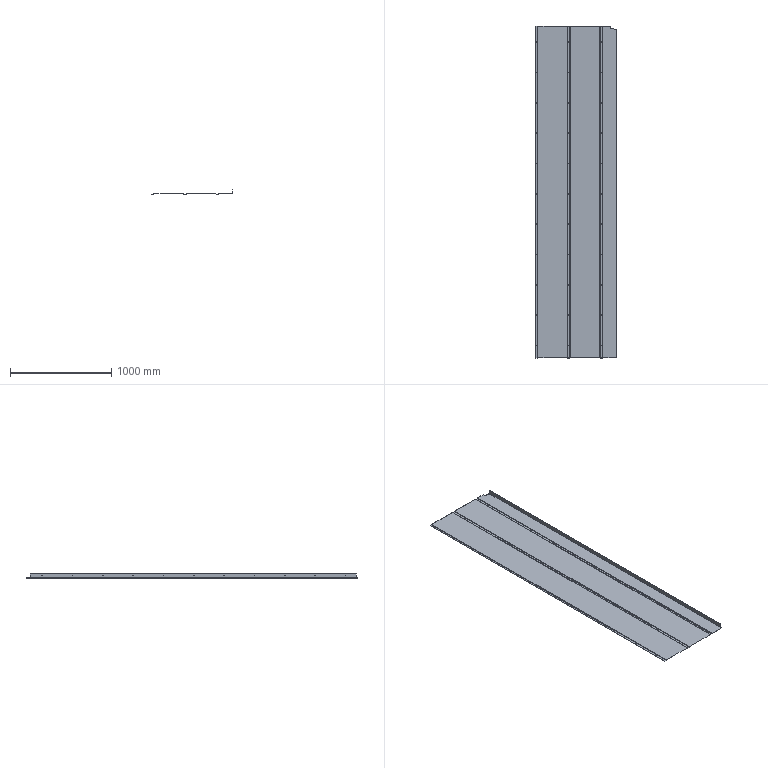Part | STEP file | TS-S84 | 1 solid | 191 faces | box 800 x 3283 x 43 mm | volume 3320511 mm3 | cylinder 113 | plane 78 | commonest cylinder face diameters 5.4 x88 0.4 x11 2.8 x11 10 x1 14 x1 16 x1